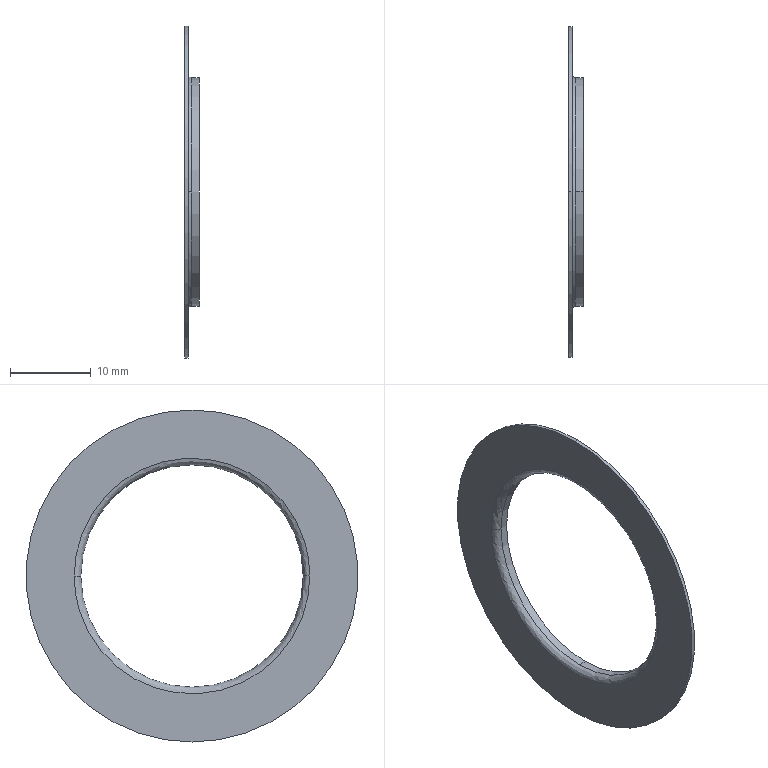Part | STEP file | Microwave Drying Flat Conveyor-inafag_ucfl204_62o9y6gnj3059x015y4y3bh4_10 | 1 solid | 13 faces | box 1.812 x 41.16 x 41.16 mm | volume 343.087 mm3 | cylinder 6 | spline 4 | plane 3 | commonest cylinder face diameters 27.56 x2 28.383 x2 41.16 x2